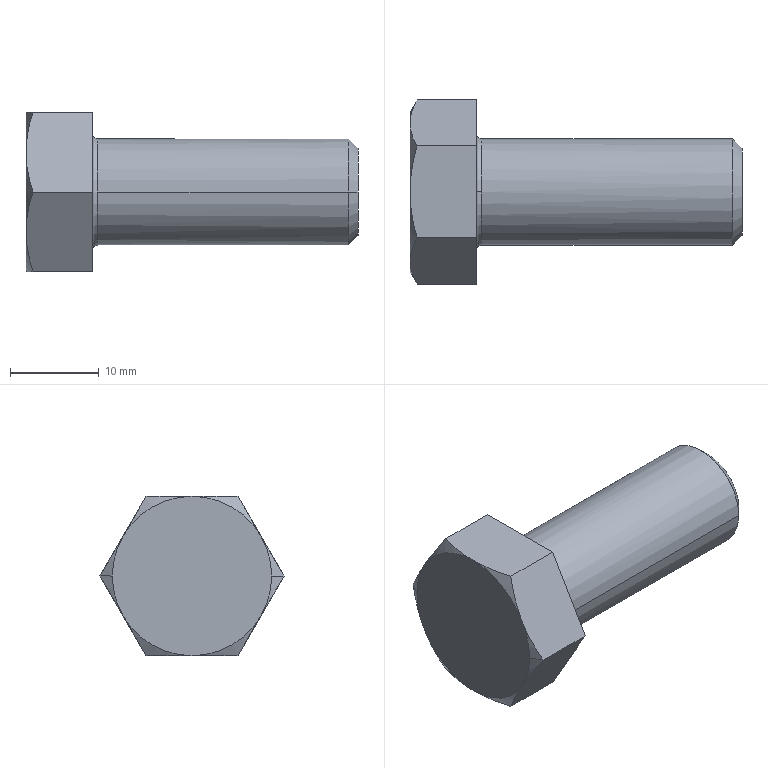Part | STEP file | KS B 1002 - C  M 12 x 30 | 1 solid | 23 faces | box 37.5 x 20.785 x 18 mm | volume 5474 mm3 | cone 10 | plane 9 | torus 2 | cylinder 2 | commonest cylinder face diameters 12 x2